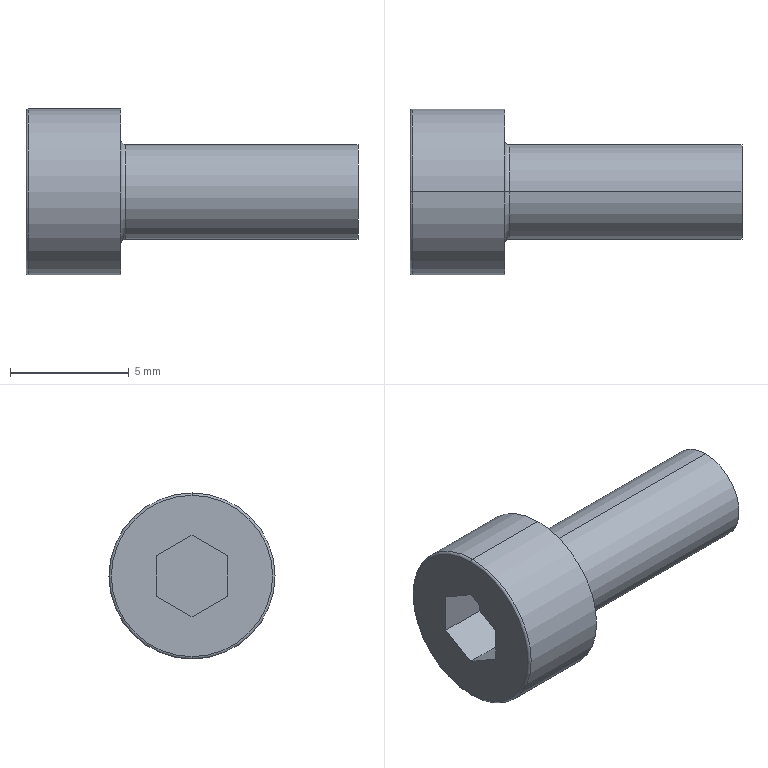Part | SolidWorks | features BlendCut 1, Cut 1, Fillet 1, LPattern 1, RevCut 1, Revolution 1 | 1 solid | 18 faces | box 14 x 7 x 7 mm | volume 264.293 mm3 | plane 10 | torus 4 | cylinder 4 | commonest cylinder face diameters 4 x2 7 x2
STEP:
#1=CARTESIAN_POINT('',(0.,0.,3.4));
#2=VERTEX_POINT('',#1);
#3=CARTESIAN_POINT('',(0.,0.,-3.4));
#4=VERTEX_POINT('',#3);
#5=CARTESIAN_POINT('',(0.,0.,0.));
#6=DIRECTION('',(-1.,0.,0.));
#7=DIRECTION('',(0.,0.,-1.));
#8=AXIS2_PLACEMENT_3D('',#5,#6,#7);
#9=CIRCLE('',#8,3.4);
#10=EDGE_CURVE('',#2,#4,#9,.T.);
#11=ORIENTED_EDGE('',*,*,#10,.F.);
#12=CARTESIAN_POINT('',(0.1,0.,3.5));
#13=VERTEX_POINT('',#12);
#14=CARTESIAN_POINT('',(0.1,0.,3.4));
#15=DIRECTION('',(0.,1.,0.));
#16=DIRECTION('',(0.,0.,1.));
#17=AXIS2_PLACEMENT_3D('',#14,#15,#16);
#18=CIRCLE('',#17,0.1);
#19=EDGE_CURVE('',#2,#13,#18,.T.);
#20=ORIENTED_EDGE('',*,*,#19,.T.);
#21=CARTESIAN_POINT('',(0.1,0.,-3.5));
#22=VERTEX_POINT('',#21);
#23=CARTESIAN_POINT('',(0.1,0.,0.));
#24=DIRECTION('',(1.,0.,0.));
#25=DIRECTION('',(0.,0.,-1.));
#26=AXIS2_PLACEMENT_3D('',#23,#24,#25);
#27=CIRCLE('',#26,3.5);
#28=EDGE_CURVE('',#22,#13,#27,.T.);
#29=ORIENTED_EDGE('',*,*,#28,.F.);
#30=CARTESIAN_POINT('',(0.1,0.,-3.4));
#31=DIRECTION('',(0.,-1.,0.));
#32=DIRECTION('',(0.,0.,-1.));
#33=AXIS2_PLACEMENT_3D('',#30,#31,#32);
#34=CIRCLE('',#33,0.1);
#35=EDGE_CURVE('',#4,#22,#34,.T.);
#36=ORIENTED_EDGE('',*,*,#35,.F.);
#37=EDGE_LOOP('',(#11,#20,#29,#36));
#38=FACE_OUTER_BOUND('',#37,.T.);
#39=CARTESIAN_POINT('',(0.1,0.,0.));
#40=DIRECTION('',(1.,0.,0.));
#41=DIRECTION('',(0.,0.,-1.));
#42=AXIS2_PLACEMENT_3D('',#39,#40,#41);
#43=TOROIDAL_SURFACE('',#42,3.4,0.1);
#44=ADVANCED_FACE('',(#38),#43,.T.);
#45=CARTESIAN_POINT('',(14.,0.,2.));
#46=VERTEX_POINT('',#45);
#47=CARTESIAN_POINT('',(14.,0.,-2.));
#48=VERTEX_POINT('',#47);
#49=CARTESIAN_POINT('',(14.,0.,0.));
#50=DIRECTION('',(-1.,0.,0.));
#51=DIRECTION('',(0.,0.,1.));
#52=AXIS2_PLACEMENT_3D('',#49,#50,#51);
#53=CIRCLE('',#52,2.);
#54=EDGE_CURVE('',#46,#48,#53,.T.);
#55=ORIENTED_EDGE('',*,*,#54,.T.);
#56=CARTESIAN_POINT('',(4.2,0.,-2.));
#57=VERTEX_POINT('',#56);
#58=CARTESIAN_POINT('',(0.,0.,-2.));
#59=DIRECTION('',(-1.,0.,0.));
#60=VECTOR('',#59,1000.);
#61=LINE('',#58,#60);
#62=EDGE_CURVE('',#48,#57,#61,.T.);
#63=ORIENTED_EDGE('',*,*,#62,.T.);
#64=CARTESIAN_POINT('',(4.2,0.,2.));
#65=VERTEX_POINT('',#64);
#66=CARTESIAN_POINT('',(4.2,0.,0.));
#67=DIRECTION('',(-1.,0.,0.));
#68=DIRECTION('',(0.,0.,1.));
#69=AXIS2_PLACEMENT_3D('',#66,#67,#68);
#70=CIRCLE('',#69,2.);
#71=EDGE_CURVE('',#65,#57,#70,.T.);
#72=ORIENTED_EDGE('',*,*,#71,.F.);
#73=CARTESIAN_POINT('',(0.,0.,2.));
#74=DIRECTION('',(-1.,0.,0.));
#75=VECTOR('',#74,1000.);
#76=LINE('',#73,#75);
#77=EDGE_CURVE('',#46,#65,#76,.T.);
#78=ORIENTED_EDGE('',*,*,#77,.F.);
#79=EDGE_LOOP('',(#55,#63,#72,#78));
#80=FACE_OUTER_BOUND('',#79,.T.);
#81=CARTESIAN_POINT('',(0.,0.,0.));
#82=DIRECTION('',(-1.,0.,0.));
#83=DIRECTION('',(0.,0.,1.));
#84=AXIS2_PLACEMENT_3D('',#81,#82,#83);
#85=CYLINDRICAL_SURFACE('',#84,2.);
#86=ADVANCED_FACE('',(#80),#85,.T.);
#87=CARTESIAN_POINT('',(4.,0.,-2.2));
#88=VERTEX_POINT('',#87);
#89=CARTESIAN_POINT('',(4.,0.,2.2));
#90=VERTEX_POINT('',#89);
#91=CARTESIAN_POINT('',(4.,0.,0.));
#92=DIRECTION('',(-1.,0.,0.));
#93=DIRECTION('',(0.,0.,1.));
#94=AXIS2_PLACEMENT_3D('',#91,#92,#93);
#95=CIRCLE('',#94,2.2);
#96=EDGE_CURVE('',#88,#90,#95,.T.);
#97=ORIENTED_EDGE('',*,*,#96,.F.);
#98=CARTESIAN_POINT('',(4.2,0.,-2.2));
#99=DIRECTION('',(0.,1.,0.));
#100=DIRECTION('',(0.,0.,1.));
#101=AXIS2_PLACEMENT_3D('',#98,#99,#100);
#102=CIRCLE('',#101,0.2);
#103=EDGE_CURVE('',#88,#57,#102,.T.);
#104=ORIENTED_EDGE('',*,*,#103,.T.);
#105=CARTESIAN_POINT('',(4.2,0.,0.));
#106=DIRECTION('',(-1.,0.,0.));
#107=DIRECTION('',(0.,0.,1.));
#108=AXIS2_PLACEMENT_3D('',#105,#106,#107);
#109=CIRCLE('',#108,2.);
#110=EDGE_CURVE('',#57,#65,#109,.T.);
#111=ORIENTED_EDGE('',*,*,#110,.T.);
#112=CARTESIAN_POINT('',(4.2,0.,2.2));
#113=DIRECTION('',(0.,-1.,0.));
#114=DIRECTION('',(0.,0.,-1.));
#115=AXIS2_PLACEMENT_3D('',#112,#113,#114);
#116=CIRCLE('',#115,0.2);
#117=EDGE_CURVE('',#90,#65,#116,.T.);
#118=ORIENTED_EDGE('',*,*,#117,.F.);
#119=EDGE_LOOP('',(#97,#104,#111,#118));
#120=FACE_OUTER_BOUND('',#119,.T.);
#121=CARTESIAN_POINT('',(4.2,0.,0.));
#122=DIRECTION('',(-1.,0.,0.));
#123=DIRECTION('',(0.,0.,1.));
#124=AXIS2_PLACEMENT_3D('',#121,#122,#123);
#125=TOROIDAL_SURFACE('',#124,2.2,0.2);
#126=ADVANCED_FACE('',(#120),#125,.F.);
#127=CARTESIAN_POINT('',(4.,0.,3.5));
#128=VERTEX_POINT('',#127);
#129=CARTESIAN_POINT('',(4.,0.,-3.5));
#130=VERTEX_POINT('',#129);
#131=CARTESIAN_POINT('',(4.,0.,0.));
#132=DIRECTION('',(-1.,0.,0.));
#133=DIRECTION('',(0.,0.,1.));
#134=AXIS2_PLACEMENT_3D('',#131,#132,#133);
#135=CIRCLE('',#134,3.5);
#136=EDGE_CURVE('',#128,#130,#135,.T.);
#137=ORIENTED_EDGE('',*,*,#136,.T.);
#138=CARTESIAN_POINT('',(0.,0.,-3.5));
#139=DIRECTION('',(-1.,0.,0.));
#140=VECTOR('',#139,1000.);
#141=LINE('',#138,#140);
#142=EDGE_CURVE('',#130,#22,#141,.T.);
#143=ORIENTED_EDGE('',*,*,#142,.T.);
#144=ORIENTED_EDGE('',*,*,#28,.T.);
#145=CARTESIAN_POINT('',(0.,0.,3.5));
#146=DIRECTION('',(-1.,0.,0.));
#147=VECTOR('',#146,1000.);
#148=LINE('',#145,#147);
#149=EDGE_CURVE('',#128,#13,#148,.T.);
#150=ORIENTED_EDGE('',*,*,#149,.F.);
#151=EDGE_LOOP('',(#137,#143,#144,#150));
#152=FACE_OUTER_BOUND('',#151,.T.);
#153=CARTESIAN_POINT('',(0.,0.,0.));
#154=DIRECTION('',(-1.,0.,0.));
#155=DIRECTION('',(0.,0.,1.));
#156=AXIS2_PLACEMENT_3D('',#153,#154,#155);
#157=CYLINDRICAL_SURFACE('',#156,3.5);
#158=ADVANCED_FACE('',(#152),#157,.T.);
#159=CARTESIAN_POINT('',(0.,0.,0.));
#160=DIRECTION('',(-1.,0.,0.));
#161=DIRECTION('',(0.,0.,-1.));
#162=AXIS2_PLACEMENT_3D('',#159,#160,#161);
#163=CIRCLE('',#162,3.4);
#164=EDGE_CURVE('',#4,#2,#163,.T.);
#165=ORIENTED_EDGE('',*,*,#164,.T.);
#166=ORIENTED_EDGE('',*,*,#10,.T.);
#167=EDGE_LOOP('',(#165,#166));
#168=FACE_OUTER_BOUND('',#167,.T.);
#169=CARTESIAN_POINT('',(0.,0.,1.72));
#170=VERTEX_POINT('',#169);
#171=CARTESIAN_POINT('',(0.,1.49,0.86));
#172=VERTEX_POINT('',#171);
#173=CARTESIAN_POINT('',(0.,0.,1.72));
#174=DIRECTION('',(0.,0.866,-0.5));
#175=VECTOR('',#174,1000.);
#176=LINE('',#173,#175);
#177=EDGE_CURVE('',#170,#172,#176,.T.);
#178=ORIENTED_EDGE('',*,*,#177,.F.);
#179=CARTESIAN_POINT('',(0.,-1.49,0.86));
#180=VERTEX_POINT('',#179);
#181=CARTESIAN_POINT('',(0.,-1.49,0.86));
#182=DIRECTION('',(0.,0.866,0.5));
#183=VECTOR('',#182,1000.);
#184=LINE('',#181,#183);
#185=EDGE_CURVE('',#180,#170,#184,.T.);
#186=ORIENTED_EDGE('',*,*,#185,.F.);
#187=CARTESIAN_POINT('',(0.,-1.49,-0.86));
#188=VERTEX_POINT('',#187);
#189=CARTESIAN_POINT('',(0.,-1.49,-0.86));
#190=DIRECTION('',(0.,0.,1.));
#191=VECTOR('',#190,1000.);
#192=LINE('',#189,#191);
#193=EDGE_CURVE('',#188,#180,#192,.T.);
#194=ORIENTED_EDGE('',*,*,#193,.F.);
#195=CARTESIAN_POINT('',(0.,0.,-1.72));
#196=VERTEX_POINT('',#195);
#197=CARTESIAN_POINT('',(0.,0.,-1.72));
#198=DIRECTION('',(0.,-0.866,0.5));
#199=VECTOR('',#198,1000.);
#200=LINE('',#197,#199);
#201=EDGE_CURVE('',#196,#188,#200,.T.);
#202=ORIENTED_EDGE('',*,*,#201,.F.);
#203=CARTESIAN_POINT('',(0.,1.49,-0.86));
#204=VERTEX_POINT('',#203);
#205=CARTESIAN_POINT('',(0.,1.49,-0.86));
#206=DIRECTION('',(0.,-0.866,-0.5));
#207=VECTOR('',#206,1000.);
#208=LINE('',#205,#207);
#209=EDGE_CURVE('',#204,#196,#208,.T.);
#210=ORIENTED_EDGE('',*,*,#209,.F.);
#211=CARTESIAN_POINT('',(0.,1.49,0.86));
#212=DIRECTION('',(0.,0.,-1.));
#213=VECTOR('',#212,1000.);
#214=LINE('',#211,#213);
#215=EDGE_CURVE('',#172,#204,#214,.T.);
#216=ORIENTED_EDGE('',*,*,#215,.F.);
#217=EDGE_LOOP('',(#178,#186,#194,#202,#210,#216));
#218=FACE_BOUND('',#217,.T.);
#219=CARTESIAN_POINT('',(0.,0.,0.));
#220=DIRECTION('',(1.,0.,0.));
#221=DIRECTION('',(0.,0.,-1.));
#222=AXIS2_PLACEMENT_3D('',#219,#220,#221);
#223=PLANE('',#222);
#224=ADVANCED_FACE('',(#168,#218),#223,.F.);
#225=ORIENTED_EDGE('',*,*,#142,.F.);
#226=CARTESIAN_POINT('',(4.,0.,0.));
#227=DIRECTION('',(-1.,0.,0.));
#228=DIRECTION('',(0.,0.,1.));
#229=AXIS2_PLACEMENT_3D('',#226,#227,#228);
#230=CIRCLE('',#229,3.5);
#231=EDGE_CURVE('',#130,#128,#230,.T.);
#232=ORIENTED_EDGE('',*,*,#231,.T.);
#233=ORIENTED_EDGE('',*,*,#149,.T.);
#234=CARTESIAN_POINT('',(0.1,0.,0.));
#235=DIRECTION('',(1.,0.,0.));
#236=DIRECTION('',(0.,0.,-1.));
#237=AXIS2_PLACEMENT_3D('',#234,#235,#236);
#238=CIRCLE('',#237,3.5);
#239=EDGE_CURVE('',#13,#22,#238,.T.);
#240=ORIENTED_EDGE('',*,*,#239,.T.);
#241=EDGE_LOOP('',(#225,#232,#233,#240));
#242=FACE_OUTER_BOUND('',#241,.T.);
#243=CARTESIAN_POINT('',(0.,0.,0.));
#244=DIRECTION('',(-1.,0.,0.));
#245=DIRECTION('',(0.,0.,1.));
#246=AXIS2_PLACEMENT_3D('',#243,#244,#245);
#247=CYLINDRICAL_SURFACE('',#246,3.5);
#248=ADVANCED_FACE('',(#242),#247,.T.);
#249=ORIENTED_EDGE('',*,*,#136,.F.);
#250=ORIENTED_EDGE('',*,*,#231,.F.);
#251=EDGE_LOOP('',(#249,#250));
#252=FACE_OUTER_BOUND('',#251,.T.);
#253=CARTESIAN_POINT('',(4.,0.,0.));
#254=DIRECTION('',(-1.,0.,0.));
#255=DIRECTION('',(0.,0.,1.));
#256=AXIS2_PLACEMENT_3D('',#253,#254,#255);
#257=CIRCLE('',#256,2.2);
#258=EDGE_CURVE('',#90,#88,#257,.T.);
#259=ORIENTED_EDGE('',*,*,#258,.T.);
#260=ORIENTED_EDGE('',*,*,#96,.T.);
#261=EDGE_LOOP('',(#259,#260));
#262=FACE_BOUND('',#261,.T.);
#263=CARTESIAN_POINT('',(4.,3.5,0.));
#264=DIRECTION('',(-1.,0.,0.));
#265=DIRECTION('',(0.,0.,1.));
#266=AXIS2_PLACEMENT_3D('',#263,#264,#265);
#267=PLANE('',#266);
#268=ADVANCED_FACE('',(#252,#262),#267,.F.);
#269=ORIENTED_EDGE('',*,*,#103,.F.);
#270=ORIENTED_EDGE('',*,*,#258,.F.);
#271=ORIENTED_EDGE('',*,*,#117,.T.);
#272=ORIENTED_EDGE('',*,*,#71,.T.);
#273=EDGE_LOOP('',(#269,#270,#271,#272));
#274=FACE_OUTER_BOUND('',#273,.T.);
#275=CARTESIAN_POINT('',(4.2,0.,0.));
#276=DIRECTION('',(-1.,0.,0.));
#277=DIRECTION('',(0.,0.,1.));
#278=AXIS2_PLACEMENT_3D('',#275,#276,#277);
#279=TOROIDAL_SURFACE('',#278,2.2,0.2);
#280=ADVANCED_FACE('',(#274),#279,.F.);
#281=ORIENTED_EDGE('',*,*,#62,.F.);
#282=CARTESIAN_POINT('',(14.,0.,0.));
#283=DIRECTION('',(-1.,0.,0.));
#284=DIRECTION('',(0.,0.,1.));
#285=AXIS2_PLACEMENT_3D('',#282,#283,#284);
#286=CIRCLE('',#285,2.);
#287=EDGE_CURVE('',#48,#46,#286,.T.);
#288=ORIENTED_EDGE('',*,*,#287,.T.);
#289=ORIENTED_EDGE('',*,*,#77,.T.);
#290=ORIENTED_EDGE('',*,*,#110,.F.);
#291=EDGE_LOOP('',(#281,#288,#289,#290));
#292=FACE_OUTER_BOUND('',#291,.T.);
#293=CARTESIAN_POINT('',(0.,0.,0.));
#294=DIRECTION('',(-1.,0.,0.));
#295=DIRECTION('',(0.,0.,1.));
#296=AXIS2_PLACEMENT_3D('',#293,#294,#295);
#297=CYLINDRICAL_SURFACE('',#296,2.);
#298=ADVANCED_FACE('',(#292),#297,.T.);
#299=ORIENTED_EDGE('',*,*,#54,.F.);
#300=ORIENTED_EDGE('',*,*,#287,.F.);
#301=EDGE_LOOP('',(#299,#300));
#302=FACE_OUTER_BOUND('',#301,.T.);
#303=CARTESIAN_POINT('',(14.,2.,0.));
#304=DIRECTION('',(-1.,0.,0.));
#305=DIRECTION('',(0.,0.,1.));
#306=AXIS2_PLACEMENT_3D('',#303,#304,#305);
#307=PLANE('',#306);
#308=ADVANCED_FACE('',(#302),#307,.F.);
#309=ORIENTED_EDGE('',*,*,#185,.T.);
#310=CARTESIAN_POINT('',(2.,0.,1.72));
#311=VERTEX_POINT('',#310);
#312=CARTESIAN_POINT('',(2.,0.,1.72));
#313=DIRECTION('',(-1.,0.,0.));
#314=VECTOR('',#313,1000.);
#315=LINE('',#312,#314);
#316=EDGE_CURVE('',#311,#170,#315,.T.);
#317=ORIENTED_EDGE('',*,*,#316,.F.);
#318=CARTESIAN_POINT('',(2.,-1.49,0.86));
#319=VERTEX_POINT('',#318);
#320=CARTESIAN_POINT('',(2.,-1.49,0.86));
#321=DIRECTION('',(0.,0.866,0.5));
#322=VECTOR('',#321,1000.);
#323=LINE('',#320,#322);
#324=EDGE_CURVE('',#319,#311,#323,.T.);
#325=ORIENTED_EDGE('',*,*,#324,.F.);
#326=CARTESIAN_POINT('',(2.,-1.49,0.86));
#327=DIRECTION('',(-1.,0.,0.));
#328=VECTOR('',#327,1000.);
#329=LINE('',#326,#328);
#330=EDGE_CURVE('',#319,#180,#329,.T.);
#331=ORIENTED_EDGE('',*,*,#330,.T.);
#332=EDGE_LOOP('',(#309,#317,#325,#331));
#333=FACE_OUTER_BOUND('',#332,.T.);
#334=CARTESIAN_POINT('',(2.,-1.49,0.86));
#335=DIRECTION('',(0.,-0.5,0.866));
#336=DIRECTION('',(0.,-0.866,-0.5));
#337=AXIS2_PLACEMENT_3D('',#334,#335,#336);
#338=PLANE('',#337);
#339=ADVANCED_FACE('',(#333),#338,.F.);
#340=ORIENTED_EDGE('',*,*,#193,.T.);
#341=ORIENTED_EDGE('',*,*,#330,.F.);
#342=CARTESIAN_POINT('',(2.,-1.49,-0.86));
#343=VERTEX_POINT('',#342);
#344=CARTESIAN_POINT('',(2.,-1.49,-0.86));
#345=DIRECTION('',(0.,0.,1.));
#346=VECTOR('',#345,1000.);
#347=LINE('',#344,#346);
#348=EDGE_CURVE('',#343,#319,#347,.T.);
#349=ORIENTED_EDGE('',*,*,#348,.F.);
#350=CARTESIAN_POINT('',(2.,-1.49,-0.86));
#351=DIRECTION('',(-1.,0.,0.));
#352=VECTOR('',#351,1000.);
#353=LINE('',#350,#352);
#354=EDGE_CURVE('',#343,#188,#353,.T.);
#355=ORIENTED_EDGE('',*,*,#354,.T.);
#356=EDGE_LOOP('',(#340,#341,#349,#355));
#357=FACE_OUTER_BOUND('',#356,.T.);
#358=CARTESIAN_POINT('',(2.,-1.49,-0.86));
#359=DIRECTION('',(0.,-1.,0.));
#360=DIRECTION('',(0.,0.,-1.));
#361=AXIS2_PLACEMENT_3D('',#358,#359,#360);
#362=PLANE('',#361);
#363=ADVANCED_FACE('',(#357),#362,.F.);
#364=ORIENTED_EDGE('',*,*,#201,.T.);
#365=ORIENTED_EDGE('',*,*,#354,.F.);
#366=CARTESIAN_POINT('',(2.,0.,-1.72));
#367=VERTEX_POINT('',#366);
#368=CARTESIAN_POINT('',(2.,0.,-1.72));
#369=DIRECTION('',(0.,-0.866,0.5));
#370=VECTOR('',#369,1000.);
#371=LINE('',#368,#370);
#372=EDGE_CURVE('',#367,#343,#371,.T.);
#373=ORIENTED_EDGE('',*,*,#372,.F.);
#374=CARTESIAN_POINT('',(2.,0.,-1.72));
#375=DIRECTION('',(-1.,0.,0.));
#376=VECTOR('',#375,1000.);
#377=LINE('',#374,#376);
#378=EDGE_CURVE('',#367,#196,#377,.T.);
#379=ORIENTED_EDGE('',*,*,#378,.T.);
#380=EDGE_LOOP('',(#364,#365,#373,#379));
#381=FACE_OUTER_BOUND('',#380,.T.);
#382=CARTESIAN_POINT('',(2.,0.,-1.72));
#383=DIRECTION('',(0.,-0.5,-0.866));
#384=DIRECTION('',(0.,0.866,-0.5));
#385=AXIS2_PLACEMENT_3D('',#382,#383,#384);
#386=PLANE('',#385);
#387=ADVANCED_FACE('',(#381),#386,.F.);
#388=ORIENTED_EDGE('',*,*,#209,.T.);
#389=ORIENTED_EDGE('',*,*,#378,.F.);
#390=CARTESIAN_POINT('',(2.,1.49,-0.86));
#391=VERTEX_POINT('',#390);
#392=CARTESIAN_POINT('',(2.,1.49,-0.86));
#393=DIRECTION('',(0.,-0.866,-0.5));
#394=VECTOR('',#393,1000.);
#395=LINE('',#392,#394);
#396=EDGE_CURVE('',#391,#367,#395,.T.);
#397=ORIENTED_EDGE('',*,*,#396,.F.);
#398=CARTESIAN_POINT('',(2.,1.49,-0.86));
#399=DIRECTION('',(-1.,0.,0.));
#400=VECTOR('',#399,1000.);
#401=LINE('',#398,#400);
#402=EDGE_CURVE('',#391,#204,#401,.T.);
#403=ORIENTED_EDGE('',*,*,#402,.T.);
#404=EDGE_LOOP('',(#388,#389,#397,#403));
#405=FACE_OUTER_BOUND('',#404,.T.);
#406=CARTESIAN_POINT('',(2.,1.49,-0.86));
#407=DIRECTION('',(0.,0.5,-0.866));
#408=DIRECTION('',(0.,0.866,0.5));
#409=AXIS2_PLACEMENT_3D('',#406,#407,#408);
#410=PLANE('',#409);
#411=ADVANCED_FACE('',(#405),#410,.F.);
#412=ORIENTED_EDGE('',*,*,#215,.T.);
#413=ORIENTED_EDGE('',*,*,#402,.F.);
#414=CARTESIAN_POINT('',(2.,1.49,0.86));
#415=VERTEX_POINT('',#414);
#416=CARTESIAN_POINT('',(2.,1.49,0.86));
#417=DIRECTION('',(0.,0.,-1.));
#418=VECTOR('',#417,1000.);
#419=LINE('',#416,#418);
#420=EDGE_CURVE('',#415,#391,#419,.T.);
#421=ORIENTED_EDGE('',*,*,#420,.F.);
#422=CARTESIAN_POINT('',(2.,1.49,0.86));
#423=DIRECTION('',(-1.,0.,0.));
#424=VECTOR('',#423,1000.);
#425=LINE('',#422,#424);
#426=EDGE_CURVE('',#415,#172,#425,.T.);
#427=ORIENTED_EDGE('',*,*,#426,.T.);
#428=EDGE_LOOP('',(#412,#413,#421,#427));
#429=FACE_OUTER_BOUND('',#428,.T.);
#430=CARTESIAN_POINT('',(2.,1.49,0.86));
#431=DIRECTION('',(0.,1.,0.));
#432=DIRECTION('',(0.,0.,1.));
#433=AXIS2_PLACEMENT_3D('',#430,#431,#432);
#434=PLANE('',#433);
#435=ADVANCED_FACE('',(#429),#434,.F.);
#436=ORIENTED_EDGE('',*,*,#177,.T.);
#437=ORIENTED_EDGE('',*,*,#426,.F.);
#438=CARTESIAN_POINT('',(2.,0.,1.72));
#439=DIRECTION('',(0.,0.866,-0.5));
#440=VECTOR('',#439,1000.);
#441=LINE('',#438,#440);
#442=EDGE_CURVE('',#311,#415,#441,.T.);
#443=ORIENTED_EDGE('',*,*,#442,.F.);
#444=ORIENTED_EDGE('',*,*,#316,.T.);
#445=EDGE_LOOP('',(#436,#437,#443,#444));
#446=FACE_OUTER_BOUND('',#445,.T.);
#447=CARTESIAN_POINT('',(2.,0.,1.72));
#448=DIRECTION('',(0.,0.5,0.866));
#449=DIRECTION('',(0.,-0.866,0.5));
#450=AXIS2_PLACEMENT_3D('',#447,#448,#449);
#451=PLANE('',#450);
#452=ADVANCED_FACE('',(#446),#451,.F.);
#453=ORIENTED_EDGE('',*,*,#324,.T.);
#454=ORIENTED_EDGE('',*,*,#442,.T.);
#455=ORIENTED_EDGE('',*,*,#420,.T.);
#456=ORIENTED_EDGE('',*,*,#396,.T.);
#457=ORIENTED_EDGE('',*,*,#372,.T.);
#458=ORIENTED_EDGE('',*,*,#348,.T.);
#459=EDGE_LOOP('',(#453,#454,#455,#456,#457,#458));
#460=FACE_OUTER_BOUND('',#459,.T.);
#461=CARTESIAN_POINT('',(2.,1.49,2.58));
#462=DIRECTION('',(-1.,0.,0.));
#463=DIRECTION('',(0.,0.,1.));
#464=AXIS2_PLACEMENT_3D('',#461,#462,#463);
#465=PLANE('',#464);
#466=ADVANCED_FACE('',(#460),#465,.T.);
#467=ORIENTED_EDGE('',*,*,#19,.F.);
#468=ORIENTED_EDGE('',*,*,#164,.F.);
#469=ORIENTED_EDGE('',*,*,#35,.T.);
#470=ORIENTED_EDGE('',*,*,#239,.F.);
#471=EDGE_LOOP('',(#467,#468,#469,#470));
#472=FACE_OUTER_BOUND('',#471,.T.);
#473=CARTESIAN_POINT('',(0.1,0.,0.));
#474=DIRECTION('',(1.,0.,0.));
#475=DIRECTION('',(0.,0.,-1.));
#476=AXIS2_PLACEMENT_3D('',#473,#474,#475);
#477=TOROIDAL_SURFACE('',#476,3.4,0.1);
#478=ADVANCED_FACE('',(#472),#477,.T.);
#479=CLOSED_SHELL('',(#44,#86,#126,#158,#224,#248,#268,#280,#298,#308,#339,#363,#387,#411,#435,#452,#466,#478));
#480=MANIFOLD_SOLID_BREP('',#479);
#481=CARTESIAN_POINT('',(0.,0.,0.));
#482=DIRECTION('',(0.,0.,1.));
#483=DIRECTION('',(1.,0.,0.));
#484=AXIS2_PLACEMENT_3D('',#481,#482,#483);
#485=(LENGTH_UNIT()NAMED_UNIT(*)SI_UNIT(.MILLI.,.METRE.));
#486=UNCERTAINTY_MEASURE_WITH_UNIT(LENGTH_MEASURE(0.00001),#485,'','');
#487=(NAMED_UNIT(*)PLANE_ANGLE_UNIT()SI_UNIT($,.RADIAN.));
#488=(NAMED_UNIT(*)SI_UNIT($,.STERADIAN.)SOLID_ANGLE_UNIT());
#489=(GEOMETRIC_REPRESENTATION_CONTEXT(3)GLOBAL_UNCERTAINTY_ASSIGNED_CONTEXT((#486))GLOBAL_UNIT_ASSIGNED_CONTEXT((#485,#487,#488))REPRESENTATION_CONTEXT('',''));
#490=ADVANCED_BREP_SHAPE_REPRESENTATION('',(#480,#484),#489);